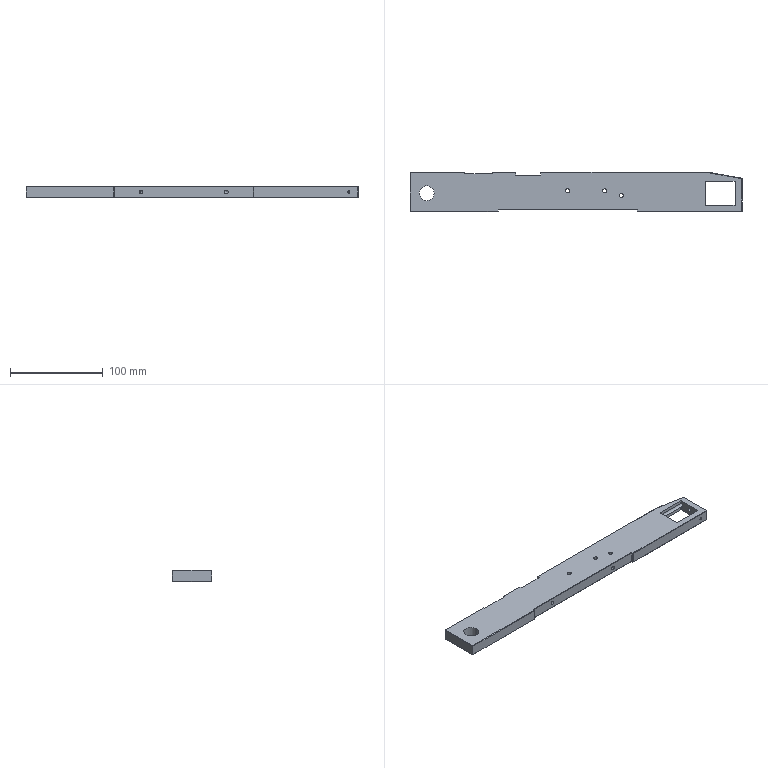Part | NX | features BREP 1 | 1 solid | 178 faces | box 358 x 42.5 x 12 mm | volume 159937 mm3 | plane 70 | cylinder 68 | cone 40 | commonest cylinder face diameters 3.3 x26 1 x8 4.2 x8 5 x8 4.3 x4 6 x4